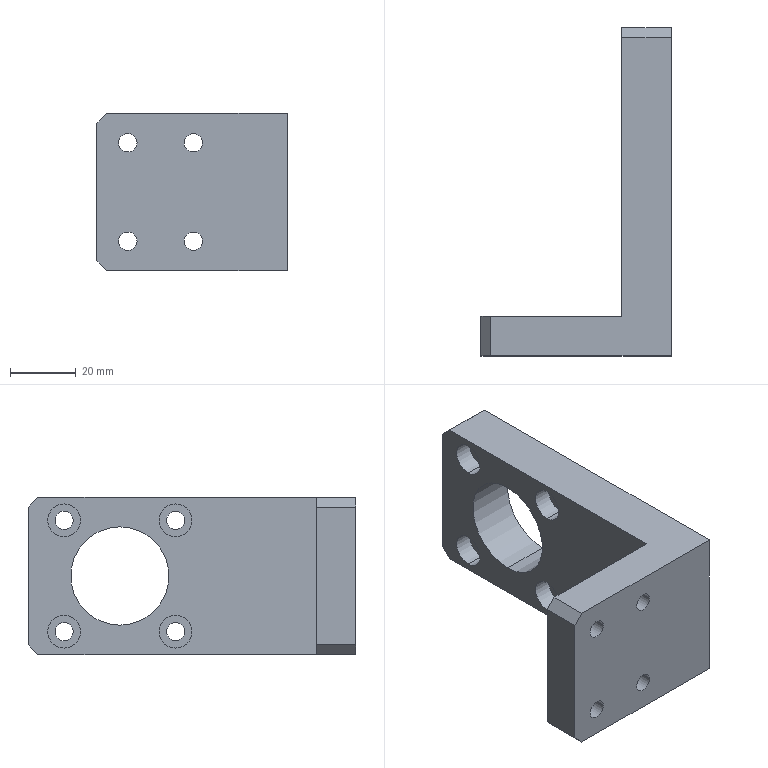Part | SolidWorks | features ICE 2, Chamfer 1, Extrusion 1, HoleWzd 1 | 1 solid | 42 faces | box 58 x 100 x 48 mm | volume 82065 mm3 | cylinder 26 | plane 16 | commonest cylinder face diameters 5.5 x8 5.6 x8 10 x8 30 x2
STEP:
#1=CARTESIAN_POINT('',(-20.01,-33.853,9.));
#2=VERTEX_POINT('',#1);
#3=CARTESIAN_POINT('',(-25.61,-33.853,9.));
#4=VERTEX_POINT('',#3);
#5=CARTESIAN_POINT('',(-22.81,-33.853,9.));
#6=DIRECTION('',(0.,1.,0.));
#7=DIRECTION('',(0.,0.,1.));
#8=AXIS2_PLACEMENT_3D('',#5,#6,#7);
#9=CIRCLE('',#8,2.8);
#10=EDGE_CURVE('',#2,#4,#9,.T.);
#11=ORIENTED_EDGE('',*,*,#10,.F.);
#12=CARTESIAN_POINT('',(-20.01,-21.853,9.));
#13=VERTEX_POINT('',#12);
#14=CARTESIAN_POINT('',(-20.01,-69.853,9.));
#15=DIRECTION('',(0.,1.,0.));
#16=VECTOR('',#15,1000.);
#17=LINE('',#14,#16);
#18=EDGE_CURVE('',#2,#13,#17,.T.);
#19=ORIENTED_EDGE('',*,*,#18,.T.);
#20=CARTESIAN_POINT('',(-25.61,-21.853,9.));
#21=VERTEX_POINT('',#20);
#22=CARTESIAN_POINT('',(-22.81,-21.853,9.));
#23=DIRECTION('',(0.,1.,0.));
#24=DIRECTION('',(-1.,0.,0.));
#25=AXIS2_PLACEMENT_3D('',#22,#23,#24);
#26=CIRCLE('',#25,2.8);
#27=EDGE_CURVE('',#13,#21,#26,.T.);
#28=ORIENTED_EDGE('',*,*,#27,.T.);
#29=CARTESIAN_POINT('',(-25.61,-69.853,9.));
#30=DIRECTION('',(0.,1.,0.));
#31=VECTOR('',#30,1000.);
#32=LINE('',#29,#31);
#33=EDGE_CURVE('',#4,#21,#32,.T.);
#34=ORIENTED_EDGE('',*,*,#33,.F.);
#35=EDGE_LOOP('',(#11,#19,#28,#34));
#36=FACE_OUTER_BOUND('',#35,.T.);
#37=CARTESIAN_POINT('',(-22.81,-69.853,9.));
#38=DIRECTION('',(0.,1.,0.));
#39=DIRECTION('',(-1.,0.,0.));
#40=AXIS2_PLACEMENT_3D('',#37,#38,#39);
#41=CYLINDRICAL_SURFACE('',#40,2.8);
#42=ADVANCED_FACE('',(#36),#41,.F.);
#43=CARTESIAN_POINT('',(-40.01,-33.853,39.));
#44=VERTEX_POINT('',#43);
#45=CARTESIAN_POINT('',(-45.61,-33.853,39.));
#46=VERTEX_POINT('',#45);
#47=CARTESIAN_POINT('',(-42.81,-33.853,39.));
#48=DIRECTION('',(0.,1.,0.));
#49=DIRECTION('',(0.,0.,1.));
#50=AXIS2_PLACEMENT_3D('',#47,#48,#49);
#51=CIRCLE('',#50,2.8);
#52=EDGE_CURVE('',#44,#46,#51,.T.);
#53=ORIENTED_EDGE('',*,*,#52,.F.);
#54=CARTESIAN_POINT('',(-40.01,-21.853,39.));
#55=VERTEX_POINT('',#54);
#56=CARTESIAN_POINT('',(-40.01,-69.853,39.));
#57=DIRECTION('',(0.,1.,0.));
#58=VECTOR('',#57,1000.);
#59=LINE('',#56,#58);
#60=EDGE_CURVE('',#44,#55,#59,.T.);
#61=ORIENTED_EDGE('',*,*,#60,.T.);
#62=CARTESIAN_POINT('',(-45.61,-21.853,39.));
#63=VERTEX_POINT('',#62);
#64=CARTESIAN_POINT('',(-42.81,-21.853,39.));
#65=DIRECTION('',(0.,1.,0.));
#66=DIRECTION('',(-1.,0.,0.));
#67=AXIS2_PLACEMENT_3D('',#64,#65,#66);
#68=CIRCLE('',#67,2.8);
#69=EDGE_CURVE('',#55,#63,#68,.T.);
#70=ORIENTED_EDGE('',*,*,#69,.T.);
#71=CARTESIAN_POINT('',(-45.61,-69.853,39.));
#72=DIRECTION('',(0.,1.,0.));
#73=VECTOR('',#72,1000.);
#74=LINE('',#71,#73);
#75=EDGE_CURVE('',#46,#63,#74,.T.);
#76=ORIENTED_EDGE('',*,*,#75,.F.);
#77=EDGE_LOOP('',(#53,#61,#70,#76));
#78=FACE_OUTER_BOUND('',#77,.T.);
#79=CARTESIAN_POINT('',(-42.81,-69.853,39.));
#80=DIRECTION('',(0.,1.,0.));
#81=DIRECTION('',(-1.,0.,0.));
#82=AXIS2_PLACEMENT_3D('',#79,#80,#81);
#83=CYLINDRICAL_SURFACE('',#82,2.8);
#84=ADVANCED_FACE('',(#78),#83,.F.);
#85=CARTESIAN_POINT('',(-20.01,-33.853,39.));
#86=VERTEX_POINT('',#85);
#87=CARTESIAN_POINT('',(-25.61,-33.853,39.));
#88=VERTEX_POINT('',#87);
#89=CARTESIAN_POINT('',(-22.81,-33.853,39.));
#90=DIRECTION('',(0.,1.,0.));
#91=DIRECTION('',(0.,0.,1.));
#92=AXIS2_PLACEMENT_3D('',#89,#90,#91);
#93=CIRCLE('',#92,2.8);
#94=EDGE_CURVE('',#86,#88,#93,.T.);
#95=ORIENTED_EDGE('',*,*,#94,.F.);
#96=CARTESIAN_POINT('',(-20.01,-21.853,39.));
#97=VERTEX_POINT('',#96);
#98=CARTESIAN_POINT('',(-20.01,-69.853,39.));
#99=DIRECTION('',(0.,1.,0.));
#100=VECTOR('',#99,1000.);
#101=LINE('',#98,#100);
#102=EDGE_CURVE('',#86,#97,#101,.T.);
#103=ORIENTED_EDGE('',*,*,#102,.T.);
#104=CARTESIAN_POINT('',(-25.61,-21.853,39.));
#105=VERTEX_POINT('',#104);
#106=CARTESIAN_POINT('',(-22.81,-21.853,39.));
#107=DIRECTION('',(0.,1.,0.));
#108=DIRECTION('',(-1.,0.,0.));
#109=AXIS2_PLACEMENT_3D('',#106,#107,#108);
#110=CIRCLE('',#109,2.8);
#111=EDGE_CURVE('',#97,#105,#110,.T.);
#112=ORIENTED_EDGE('',*,*,#111,.T.);
#113=CARTESIAN_POINT('',(-25.61,-69.853,39.));
#114=DIRECTION('',(0.,1.,0.));
#115=VECTOR('',#114,1000.);
#116=LINE('',#113,#115);
#117=EDGE_CURVE('',#88,#105,#116,.T.);
#118=ORIENTED_EDGE('',*,*,#117,.F.);
#119=EDGE_LOOP('',(#95,#103,#112,#118));
#120=FACE_OUTER_BOUND('',#119,.T.);
#121=CARTESIAN_POINT('',(-22.81,-69.853,39.));
#122=DIRECTION('',(0.,1.,0.));
#123=DIRECTION('',(-1.,0.,0.));
#124=AXIS2_PLACEMENT_3D('',#121,#122,#123);
#125=CYLINDRICAL_SURFACE('',#124,2.8);
#126=ADVANCED_FACE('',(#120),#125,.F.);
#127=CARTESIAN_POINT('',(-40.01,-33.853,9.));
#128=VERTEX_POINT('',#127);
#129=CARTESIAN_POINT('',(-45.61,-33.853,9.));
#130=VERTEX_POINT('',#129);
#131=CARTESIAN_POINT('',(-42.81,-33.853,9.));
#132=DIRECTION('',(0.,1.,0.));
#133=DIRECTION('',(0.,0.,1.));
#134=AXIS2_PLACEMENT_3D('',#131,#132,#133);
#135=CIRCLE('',#134,2.8);
#136=EDGE_CURVE('',#128,#130,#135,.T.);
#137=ORIENTED_EDGE('',*,*,#136,.F.);
#138=CARTESIAN_POINT('',(-40.01,-21.853,9.));
#139=VERTEX_POINT('',#138);
#140=CARTESIAN_POINT('',(-40.01,-69.853,9.));
#141=DIRECTION('',(0.,1.,0.));
#142=VECTOR('',#141,1000.);
#143=LINE('',#140,#142);
#144=EDGE_CURVE('',#128,#139,#143,.T.);
#145=ORIENTED_EDGE('',*,*,#144,.T.);
#146=CARTESIAN_POINT('',(-45.61,-21.853,9.));
#147=VERTEX_POINT('',#146);
#148=CARTESIAN_POINT('',(-42.81,-21.853,9.));
#149=DIRECTION('',(0.,1.,0.));
#150=DIRECTION('',(-1.,0.,0.));
#151=AXIS2_PLACEMENT_3D('',#148,#149,#150);
#152=CIRCLE('',#151,2.8);
#153=EDGE_CURVE('',#139,#147,#152,.T.);
#154=ORIENTED_EDGE('',*,*,#153,.T.);
#155=CARTESIAN_POINT('',(-45.61,-69.853,9.));
#156=DIRECTION('',(0.,1.,0.));
#157=VECTOR('',#156,1000.);
#158=LINE('',#155,#157);
#159=EDGE_CURVE('',#130,#147,#158,.T.);
#160=ORIENTED_EDGE('',*,*,#159,.F.);
#161=EDGE_LOOP('',(#137,#145,#154,#160));
#162=FACE_OUTER_BOUND('',#161,.T.);
#163=CARTESIAN_POINT('',(-42.81,-69.853,9.));
#164=DIRECTION('',(0.,1.,0.));
#165=DIRECTION('',(-1.,0.,0.));
#166=AXIS2_PLACEMENT_3D('',#163,#164,#165);
#167=CYLINDRICAL_SURFACE('',#166,2.8);
#168=ADVANCED_FACE('',(#162),#167,.F.);
#169=CARTESIAN_POINT('',(-3.547,55.147,2.));
#170=VERTEX_POINT('',#169);
#171=CARTESIAN_POINT('',(-3.547,55.147,12.));
#172=VERTEX_POINT('',#171);
#173=CARTESIAN_POINT('',(-3.547,55.147,7.));
#174=DIRECTION('',(-1.,0.,0.));
#175=DIRECTION('',(0.,0.,1.));
#176=AXIS2_PLACEMENT_3D('',#173,#174,#175);
#177=CIRCLE('',#176,5.);
#178=EDGE_CURVE('',#170,#172,#177,.T.);
#179=ORIENTED_EDGE('',*,*,#178,.F.);
#180=CARTESIAN_POINT('',(-9.247,55.147,2.));
#181=VERTEX_POINT('',#180);
#182=CARTESIAN_POINT('',(-9.247,55.147,2.));
#183=DIRECTION('',(-1.,0.,0.));
#184=VECTOR('',#183,1000.);
#185=LINE('',#182,#184);
#186=EDGE_CURVE('',#170,#181,#185,.T.);
#187=ORIENTED_EDGE('',*,*,#186,.T.);
#188=CARTESIAN_POINT('',(-9.247,55.147,12.));
#189=VERTEX_POINT('',#188);
#190=CARTESIAN_POINT('',(-9.247,55.147,7.));
#191=DIRECTION('',(-1.,0.,0.));
#192=DIRECTION('',(0.,0.,1.));
#193=AXIS2_PLACEMENT_3D('',#190,#191,#192);
#194=CIRCLE('',#193,5.);
#195=EDGE_CURVE('',#181,#189,#194,.T.);
#196=ORIENTED_EDGE('',*,*,#195,.T.);
#197=CARTESIAN_POINT('',(-9.247,55.147,12.));
#198=DIRECTION('',(-1.,0.,0.));
#199=VECTOR('',#198,1000.);
#200=LINE('',#197,#199);
#201=EDGE_CURVE('',#172,#189,#200,.T.);
#202=ORIENTED_EDGE('',*,*,#201,.F.);
#203=EDGE_LOOP('',(#179,#187,#196,#202));
#204=FACE_OUTER_BOUND('',#203,.T.);
#205=CARTESIAN_POINT('',(-9.247,55.147,7.));
#206=DIRECTION('',(-1.,0.,0.));
#207=DIRECTION('',(0.,0.,1.));
#208=AXIS2_PLACEMENT_3D('',#205,#206,#207);
#209=CYLINDRICAL_SURFACE('',#208,5.);
#210=ADVANCED_FACE('',(#204),#209,.F.);
#211=CARTESIAN_POINT('',(5.753,55.147,4.25));
#212=VERTEX_POINT('',#211);
#213=CARTESIAN_POINT('',(5.753,55.147,9.75));
#214=VERTEX_POINT('',#213);
#215=CARTESIAN_POINT('',(5.753,55.147,7.));
#216=DIRECTION('',(-1.,0.,0.));
#217=DIRECTION('',(0.,0.,1.));
#218=AXIS2_PLACEMENT_3D('',#215,#216,#217);
#219=CIRCLE('',#218,2.75);
#220=EDGE_CURVE('',#212,#214,#219,.T.);
#221=ORIENTED_EDGE('',*,*,#220,.F.);
#222=CARTESIAN_POINT('',(-3.547,55.147,4.25));
#223=VERTEX_POINT('',#222);
#224=CARTESIAN_POINT('',(-9.247,55.147,4.25));
#225=DIRECTION('',(-1.,0.,0.));
#226=VECTOR('',#225,1000.);
#227=LINE('',#224,#226);
#228=EDGE_CURVE('',#212,#223,#227,.T.);
#229=ORIENTED_EDGE('',*,*,#228,.T.);
#230=CARTESIAN_POINT('',(-3.547,55.147,9.75));
#231=VERTEX_POINT('',#230);
#232=CARTESIAN_POINT('',(-3.547,55.147,7.));
#233=DIRECTION('',(-1.,0.,0.));
#234=DIRECTION('',(0.,0.,1.));
#235=AXIS2_PLACEMENT_3D('',#232,#233,#234);
#236=CIRCLE('',#235,2.75);
#237=EDGE_CURVE('',#223,#231,#236,.T.);
#238=ORIENTED_EDGE('',*,*,#237,.T.);
#239=CARTESIAN_POINT('',(-9.247,55.147,9.75));
#240=DIRECTION('',(-1.,0.,0.));
#241=VECTOR('',#240,1000.);
#242=LINE('',#239,#241);
#243=EDGE_CURVE('',#214,#231,#242,.T.);
#244=ORIENTED_EDGE('',*,*,#243,.F.);
#245=EDGE_LOOP('',(#221,#229,#238,#244));
#246=FACE_OUTER_BOUND('',#245,.T.);
#247=CARTESIAN_POINT('',(-9.247,55.147,7.));
#248=DIRECTION('',(-1.,0.,0.));
#249=DIRECTION('',(0.,0.,1.));
#250=AXIS2_PLACEMENT_3D('',#247,#248,#249);
#251=CYLINDRICAL_SURFACE('',#250,2.75);
#252=ADVANCED_FACE('',(#246),#251,.F.);
#253=CARTESIAN_POINT('',(-3.547,55.147,36.));
#254=VERTEX_POINT('',#253);
#255=CARTESIAN_POINT('',(-3.547,55.147,46.));
#256=VERTEX_POINT('',#255);
#257=CARTESIAN_POINT('',(-3.547,55.147,41.));
#258=DIRECTION('',(-1.,0.,0.));
#259=DIRECTION('',(0.,0.,1.));
#260=AXIS2_PLACEMENT_3D('',#257,#258,#259);
#261=CIRCLE('',#260,5.);
#262=EDGE_CURVE('',#254,#256,#261,.T.);
#263=ORIENTED_EDGE('',*,*,#262,.F.);
#264=CARTESIAN_POINT('',(-9.247,55.147,36.));
#265=VERTEX_POINT('',#264);
#266=CARTESIAN_POINT('',(-9.247,55.147,36.));
#267=DIRECTION('',(-1.,0.,0.));
#268=VECTOR('',#267,1000.);
#269=LINE('',#266,#268);
#270=EDGE_CURVE('',#254,#265,#269,.T.);
#271=ORIENTED_EDGE('',*,*,#270,.T.);
#272=CARTESIAN_POINT('',(-9.247,55.147,46.));
#273=VERTEX_POINT('',#272);
#274=CARTESIAN_POINT('',(-9.247,55.147,41.));
#275=DIRECTION('',(-1.,0.,0.));
#276=DIRECTION('',(0.,0.,1.));
#277=AXIS2_PLACEMENT_3D('',#274,#275,#276);
#278=CIRCLE('',#277,5.);
#279=EDGE_CURVE('',#265,#273,#278,.T.);
#280=ORIENTED_EDGE('',*,*,#279,.T.);
#281=CARTESIAN_POINT('',(-9.247,55.147,46.));
#282=DIRECTION('',(-1.,0.,0.));
#283=VECTOR('',#282,1000.);
#284=LINE('',#281,#283);
#285=EDGE_CURVE('',#256,#273,#284,.T.);
#286=ORIENTED_EDGE('',*,*,#285,.F.);
#287=EDGE_LOOP('',(#263,#271,#280,#286));
#288=FACE_OUTER_BOUND('',#287,.T.);
#289=CARTESIAN_POINT('',(-9.247,55.147,41.));
#290=DIRECTION('',(-1.,0.,0.));
#291=DIRECTION('',(0.,0.,1.));
#292=AXIS2_PLACEMENT_3D('',#289,#290,#291);
#293=CYLINDRICAL_SURFACE('',#292,5.);
#294=ADVANCED_FACE('',(#288),#293,.F.);
#295=CARTESIAN_POINT('',(5.753,55.147,38.25));
#296=VERTEX_POINT('',#295);
#297=CARTESIAN_POINT('',(5.753,55.147,43.75));
#298=VERTEX_POINT('',#297);
#299=CARTESIAN_POINT('',(5.753,55.147,41.));
#300=DIRECTION('',(-1.,0.,0.));
#301=DIRECTION('',(0.,0.,1.));
#302=AXIS2_PLACEMENT_3D('',#299,#300,#301);
#303=CIRCLE('',#302,2.75);
#304=EDGE_CURVE('',#296,#298,#303,.T.);
#305=ORIENTED_EDGE('',*,*,#304,.F.);
#306=CARTESIAN_POINT('',(-3.547,55.147,38.25));
#307=VERTEX_POINT('',#306);
#308=CARTESIAN_POINT('',(-9.247,55.147,38.25));
#309=DIRECTION('',(-1.,0.,0.));
#310=VECTOR('',#309,1000.);
#311=LINE('',#308,#310);
#312=EDGE_CURVE('',#296,#307,#311,.T.);
#313=ORIENTED_EDGE('',*,*,#312,.T.);
#314=CARTESIAN_POINT('',(-3.547,55.147,43.75));
#315=VERTEX_POINT('',#314);
#316=CARTESIAN_POINT('',(-3.547,55.147,41.));
#317=DIRECTION('',(-1.,0.,0.));
#318=DIRECTION('',(0.,0.,1.));
#319=AXIS2_PLACEMENT_3D('',#316,#317,#318);
#320=CIRCLE('',#319,2.75);
#321=EDGE_CURVE('',#307,#315,#320,.T.);
#322=ORIENTED_EDGE('',*,*,#321,.T.);
#323=CARTESIAN_POINT('',(-9.247,55.147,43.75));
#324=DIRECTION('',(-1.,0.,0.));
#325=VECTOR('',#324,1000.);
#326=LINE('',#323,#325);
#327=EDGE_CURVE('',#298,#315,#326,.T.);
#328=ORIENTED_EDGE('',*,*,#327,.F.);
#329=EDGE_LOOP('',(#305,#313,#322,#328));
#330=FACE_OUTER_BOUND('',#329,.T.);
#331=CARTESIAN_POINT('',(-9.247,55.147,41.));
#332=DIRECTION('',(-1.,0.,0.));
#333=DIRECTION('',(0.,0.,1.));
#334=AXIS2_PLACEMENT_3D('',#331,#332,#333);
#335=CYLINDRICAL_SURFACE('',#334,2.75);
#336=ADVANCED_FACE('',(#330),#335,.F.);
#337=CARTESIAN_POINT('',(-3.547,21.147,36.));
#338=VERTEX_POINT('',#337);
#339=CARTESIAN_POINT('',(-3.547,21.147,46.));
#340=VERTEX_POINT('',#339);
#341=CARTESIAN_POINT('',(-3.547,21.147,41.));
#342=DIRECTION('',(-1.,0.,0.));
#343=DIRECTION('',(0.,0.,1.));
#344=AXIS2_PLACEMENT_3D('',#341,#342,#343);
#345=CIRCLE('',#344,5.);
#346=EDGE_CURVE('',#338,#340,#345,.T.);
#347=ORIENTED_EDGE('',*,*,#346,.F.);
#348=CARTESIAN_POINT('',(-9.247,21.147,36.));
#349=VERTEX_POINT('',#348);
#350=CARTESIAN_POINT('',(-9.247,21.147,36.));
#351=DIRECTION('',(-1.,0.,0.));
#352=VECTOR('',#351,1000.);
#353=LINE('',#350,#352);
#354=EDGE_CURVE('',#338,#349,#353,.T.);
#355=ORIENTED_EDGE('',*,*,#354,.T.);
#356=CARTESIAN_POINT('',(-9.247,21.147,46.));
#357=VERTEX_POINT('',#356);
#358=CARTESIAN_POINT('',(-9.247,21.147,41.));
#359=DIRECTION('',(-1.,0.,0.));
#360=DIRECTION('',(0.,0.,1.));
#361=AXIS2_PLACEMENT_3D('',#358,#359,#360);
#362=CIRCLE('',#361,5.);
#363=EDGE_CURVE('',#349,#357,#362,.T.);
#364=ORIENTED_EDGE('',*,*,#363,.T.);
#365=CARTESIAN_POINT('',(-9.247,21.147,46.));
#366=DIRECTION('',(-1.,0.,0.));
#367=VECTOR('',#366,1000.);
#368=LINE('',#365,#367);
#369=EDGE_CURVE('',#340,#357,#368,.T.);
#370=ORIENTED_EDGE('',*,*,#369,.F.);
#371=EDGE_LOOP('',(#347,#355,#364,#370));
#372=FACE_OUTER_BOUND('',#371,.T.);
#373=CARTESIAN_POINT('',(-9.247,21.147,41.));
#374=DIRECTION('',(-1.,0.,0.));
#375=DIRECTION('',(0.,0.,1.));
#376=AXIS2_PLACEMENT_3D('',#373,#374,#375);
#377=CYLINDRICAL_SURFACE('',#376,5.);
#378=ADVANCED_FACE('',(#372),#377,.F.);
#379=CARTESIAN_POINT('',(5.753,21.147,38.25));
#380=VERTEX_POINT('',#379);
#381=CARTESIAN_POINT('',(5.753,21.147,43.75));
#382=VERTEX_POINT('',#381);
#383=CARTESIAN_POINT('',(5.753,21.147,41.));
#384=DIRECTION('',(-1.,0.,0.));
#385=DIRECTION('',(0.,0.,1.));
#386=AXIS2_PLACEMENT_3D('',#383,#384,#385);
#387=CIRCLE('',#386,2.75);
#388=EDGE_CURVE('',#380,#382,#387,.T.);
#389=ORIENTED_EDGE('',*,*,#388,.F.);
#390=CARTESIAN_POINT('',(-3.547,21.147,38.25));
#391=VERTEX_POINT('',#390);
#392=CARTESIAN_POINT('',(-9.247,21.147,38.25));
#393=DIRECTION('',(-1.,0.,0.));
#394=VECTOR('',#393,1000.);
#395=LINE('',#392,#394);
#396=EDGE_CURVE('',#380,#391,#395,.T.);
#397=ORIENTED_EDGE('',*,*,#396,.T.);
#398=CARTESIAN_POINT('',(-3.547,21.147,43.75));
#399=VERTEX_POINT('',#398);
#400=CARTESIAN_POINT('',(-3.547,21.147,41.));
#401=DIRECTION('',(-1.,0.,0.));
#402=DIRECTION('',(0.,0.,1.));
#403=AXIS2_PLACEMENT_3D('',#400,#401,#402);
#404=CIRCLE('',#403,2.75);
#405=EDGE_CURVE('',#391,#399,#404,.T.);
#406=ORIENTED_EDGE('',*,*,#405,.T.);
#407=CARTESIAN_POINT('',(-9.247,21.147,43.75));
#408=DIRECTION('',(-1.,0.,0.));
#409=VECTOR('',#408,1000.);
#410=LINE('',#407,#409);
#411=EDGE_CURVE('',#382,#399,#410,.T.);
#412=ORIENTED_EDGE('',*,*,#411,.F.);
#413=EDGE_LOOP('',(#389,#397,#406,#412));
#414=FACE_OUTER_BOUND('',#413,.T.);
#415=CARTESIAN_POINT('',(-9.247,21.147,41.));
#416=DIRECTION('',(-1.,0.,0.));
#417=DIRECTION('',(0.,0.,1.));
#418=AXIS2_PLACEMENT_3D('',#415,#416,#417);
#419=CYLINDRICAL_SURFACE('',#418,2.75);
#420=ADVANCED_FACE('',(#414),#419,.F.);
#421=CARTESIAN_POINT('',(-3.547,21.147,2.));
#422=VERTEX_POINT('',#421);
#423=CARTESIAN_POINT('',(-3.547,21.147,12.));
#424=VERTEX_POINT('',#423);
#425=CARTESIAN_POINT('',(-3.547,21.147,7.));
#426=DIRECTION('',(-1.,0.,0.));
#427=DIRECTION('',(0.,0.,1.));
#428=AXIS2_PLACEMENT_3D('',#425,#426,#427);
#429=CIRCLE('',#428,5.);
#430=EDGE_CURVE('',#422,#424,#429,.T.);
#431=ORIENTED_EDGE('',*,*,#430,.F.);
#432=CARTESIAN_POINT('',(-9.247,21.147,2.));
#433=VERTEX_POINT('',#432);
#434=CARTESIAN_POINT('',(-9.247,21.147,2.));
#435=DIRECTION('',(-1.,0.,0.));
#436=VECTOR('',#435,1000.);
#437=LINE('',#434,#436);
#438=EDGE_CURVE('',#422,#433,#437,.T.);
#439=ORIENTED_EDGE('',*,*,#438,.T.);
#440=CARTESIAN_POINT('',(-9.247,21.147,12.));
#441=VERTEX_POINT('',#440);
#442=CARTESIAN_POINT('',(-9.247,21.147,7.));
#443=DIRECTION('',(-1.,0.,0.));
#444=DIRECTION('',(0.,0.,1.));
#445=AXIS2_PLACEMENT_3D('',#442,#443,#444);
#446=CIRCLE('',#445,5.);
#447=EDGE_CURVE('',#433,#441,#446,.T.);
#448=ORIENTED_EDGE('',*,*,#447,.T.);
#449=CARTESIAN_POINT('',(-9.247,21.147,12.));
#450=DIRECTION('',(-1.,0.,0.));
#451=VECTOR('',#450,1000.);
#452=LINE('',#449,#451);
#453=EDGE_CURVE('',#424,#441,#452,.T.);
#454=ORIENTED_EDGE('',*,*,#453,.F.);
#455=EDGE_LOOP('',(#431,#439,#448,#454));
#456=FACE_OUTER_BOUND('',#455,.T.);
#457=CARTESIAN_POINT('',(-9.247,21.147,7.));
#458=DIRECTION('',(-1.,0.,0.));
#459=DIRECTION('',(0.,0.,1.));
#460=AXIS2_PLACEMENT_3D('',#457,#458,#459);
#461=CYLINDRICAL_SURFACE('',#460,5.);
#462=ADVANCED_FACE('',(#456),#461,.F.);
#463=CARTESIAN_POINT('',(5.753,21.147,4.25));
#464=VERTEX_POINT('',#463);
#465=CARTESIAN_POINT('',(5.753,21.147,9.75));
#466=VERTEX_POINT('',#465);
#467=CARTESIAN_POINT('',(5.753,21.147,7.));
#468=DIRECTION('',(-1.,0.,0.));
#469=DIRECTION('',(0.,0.,1.));
#470=AXIS2_PLACEMENT_3D('',#467,#468,#469);
#471=CIRCLE('',#470,2.75);
#472=EDGE_CURVE('',#464,#466,#471,.T.);
#473=ORIENTED_EDGE('',*,*,#472,.F.);
#474=CARTESIAN_POINT('',(-3.547,21.147,4.25));
#475=VERTEX_POINT('',#474);
#476=CARTESIAN_POINT('',(-9.247,21.147,4.25));
#477=DIRECTION('',(-1.,0.,0.));
#478=VECTOR('',#477,1000.);
#479=LINE('',#476,#478);
#480=EDGE_CURVE('',#464,#475,#479,.T.);
#481=ORIENTED_EDGE('',*,*,#480,.T.);
#482=CARTESIAN_POINT('',(-3.547,21.147,9.75));
#483=VERTEX_POINT('',#482);
#484=CARTESIAN_POINT('',(-3.547,21.147,7.));
#485=DIRECTION('',(-1.,0.,0.));
#486=DIRECTION('',(0.,0.,1.));
#487=AXIS2_PLACEMENT_3D('',#484,#485,#486);
#488=CIRCLE('',#487,2.75);
#489=EDGE_CURVE('',#475,#483,#488,.T.);
#490=ORIENTED_EDGE('',*,*,#489,.T.);
#491=CARTESIAN_POINT('',(-9.247,21.147,9.75));
#492=DIRECTION('',(-1.,0.,0.));
#493=VECTOR('',#492,1000.);
#494=LINE('',#491,#493);
#495=EDGE_CURVE('',#466,#483,#494,.T.);
#496=ORIENTED_EDGE('',*,*,#495,.F.);
#497=EDGE_LOOP('',(#473,#481,#490,#496));
#498=FACE_OUTER_BOUND('',#497,.T.);
#499=CARTESIAN_POINT('',(-9.247,21.147,7.));
#500=DIRECTION('',(-1.,0.,0.));
#501=DIRECTION('',(0.,0.,1.));
#502=AXIS2_PLACEMENT_3D('',#499,#500,#501);
#503=CYLINDRICAL_SURFACE('',#502,2.75);
#504=ADVANCED_FACE('',(#498),#503,.F.);
#505=CARTESIAN_POINT('',(5.753,38.147,9.));
#506=VERTEX_POINT('',#505);
#507=CARTESIAN_POINT('',(5.753,38.147,39.));
#508=VERTEX_POINT('',#507);
#509=CARTESIAN_POINT('',(5.753,38.147,24.));
#510=DIRECTION('',(-1.,0.,0.));
#511=DIRECTION('',(0.,0.,1.));
#512=AXIS2_PLACEMENT_3D('',#509,#510,#511);
#513=CIRCLE('',#512,15.);
#514=EDGE_CURVE('',#506,#508,#513,.T.);
#515=ORIENTED_EDGE('',*,*,#514,.F.);
#516=CARTESIAN_POINT('',(-9.247,38.147,9.));
#517=VERTEX_POINT('',#516);
#518=CARTESIAN_POINT('',(5.753,38.147,9.));
#519=DIRECTION('',(-1.,0.,0.));
#520=VECTOR('',#519,1000.);
#521=LINE('',#518,#520);
#522=EDGE_CURVE('',#506,#517,#521,.T.);
#523=ORIENTED_EDGE('',*,*,#522,.T.);
#524=CARTESIAN_POINT('',(-9.247,38.147,39.));
#525=VERTEX_POINT('',#524);
#526=CARTESIAN_POINT('',(-9.247,38.147,24.));
#527=DIRECTION('',(-1.,0.,0.));
#528=DIRECTION('',(0.,0.,1.));
#529=AXIS2_PLACEMENT_3D('',#526,#527,#528);
#530=CIRCLE('',#529,15.);
#531=EDGE_CURVE('',#517,#525,#530,.T.);
#532=ORIENTED_EDGE('',*,*,#531,.T.);
#533=CARTESIAN_POINT('',(5.753,38.147,39.));
#534=DIRECTION('',(-1.,0.,0.));
#535=VECTOR('',#534,1000.);
#536=LINE('',#533,#535);
#537=EDGE_CURVE('',#508,#525,#536,.T.);
#538=ORIENTED_EDGE('',*,*,#537,.F.);
#539=EDGE_LOOP('',(#515,#523,#532,#538));
#540=FACE_OUTER_BOUND('',#539,.T.);
#541=CARTESIAN_POINT('',(5.753,38.147,24.));
#542=DIRECTION('',(-1.,0.,0.));
#543=DIRECTION('',(0.,0.,1.));
#544=AXIS2_PLACEMENT_3D('',#541,#542,#543);
#545=CYLINDRICAL_SURFACE('',#544,15.);
#546=ADVANCED_FACE('',(#540),#545,.F.);
#547=CARTESIAN_POINT('',(-9.247,66.147,45.));
#548=VERTEX_POINT('',#547);
#549=CARTESIAN_POINT('',(-9.247,66.147,3.));
#550=VERTEX_POINT('',#549);
#551=CARTESIAN_POINT('',(-9.247,66.147,48.));
#552=DIRECTION('',(0.,0.,-1.));
#553=VECTOR('',#552,1000.);
#554=LINE('',#551,#553);
#555=EDGE_CURVE('',#548,#550,#554,.T.);
#556=ORIENTED_EDGE('',*,*,#555,.F.);
#557=CARTESIAN_POINT('',(5.753,66.147,45.));
#558=VERTEX_POINT('',#557);
#559=CARTESIAN_POINT('',(5.753,66.147,45.));
#560=DIRECTION('',(1.,0.,0.));
#561=VECTOR('',#560,1000.);
#562=LINE('',#559,#561);
#563=EDGE_CURVE('',#548,#558,#562,.T.);
#564=ORIENTED_EDGE('',*,*,#563,.T.);
#565=CARTESIAN_POINT('',(5.753,66.147,3.));
#566=VERTEX_POINT('',#565);
#567=CARTESIAN_POINT('',(5.753,66.147,48.));
#568=DIRECTION('',(0.,0.,-1.));
#569=VECTOR('',#568,1000.);
#570=LINE('',#567,#569);
#571=EDGE_CURVE('',#558,#566,#570,.T.);
#572=ORIENTED_EDGE('',*,*,#571,.T.);
#573=CARTESIAN_POINT('',(5.753,66.147,3.));
#574=DIRECTION('',(-1.,0.,0.));
#575=VECTOR('',#574,1000.);
#576=LINE('',#573,#575);
#577=EDGE_CURVE('',#566,#550,#576,.T.);
#578=ORIENTED_EDGE('',*,*,#577,.T.);
#579=EDGE_LOOP('',(#556,#564,#572,#578));
#580=FACE_OUTER_BOUND('',#579,.T.);
#581=CARTESIAN_POINT('',(5.753,66.147,48.));
#582=DIRECTION('',(0.,-1.,0.));
#583=DIRECTION('',(0.,0.,-1.));
#584=AXIS2_PLACEMENT_3D('',#581,#582,#583);
#585=PLANE('',#584);
#586=ADVANCED_FACE('',(#580),#585,.F.);
#587=CARTESIAN_POINT('',(-9.247,55.147,7.));
#588=DIRECTION('',(-1.,0.,0.));
#589=DIRECTION('',(0.,0.,1.));
#590=AXIS2_PLACEMENT_3D('',#587,#588,#589);
#591=CIRCLE('',#590,5.);
#592=EDGE_CURVE('',#189,#181,#591,.T.);
#593=ORIENTED_EDGE('',*,*,#592,.F.);
#594=ORIENTED_EDGE('',*,*,#195,.F.);
#595=EDGE_LOOP('',(#593,#594));
#596=FACE_BOUND('',#595,.T.);
#597=CARTESIAN_POINT('',(-9.247,55.147,41.));
#598=DIRECTION('',(-1.,0.,0.));
#599=DIRECTION('',(0.,0.,1.));
#600=AXIS2_PLACEMENT_3D('',#597,#598,#599);
#601=CIRCLE('',#600,5.);
#602=EDGE_CURVE('',#273,#265,#601,.T.);
#603=ORIENTED_EDGE('',*,*,#602,.F.);
#604=ORIENTED_EDGE('',*,*,#279,.F.);
#605=EDGE_LOOP('',(#603,#604));
#606=FACE_BOUND('',#605,.T.);
#607=CARTESIAN_POINT('',(-9.247,21.147,41.));
#608=DIRECTION('',(-1.,0.,0.));
#609=DIRECTION('',(0.,0.,1.));
#610=AXIS2_PLACEMENT_3D('',#607,#608,#609);
#611=CIRCLE('',#610,5.);
#612=EDGE_CURVE('',#357,#349,#611,.T.);
#613=ORIENTED_EDGE('',*,*,#612,.F.);
#614=ORIENTED_EDGE('',*,*,#363,.F.);
#615=EDGE_LOOP('',(#613,#614));
#616=FACE_BOUND('',#615,.T.);
#617=CARTESIAN_POINT('',(-9.247,21.147,7.));
#618=DIRECTION('',(-1.,0.,0.));
#619=DIRECTION('',(0.,0.,1.));
#620=AXIS2_PLACEMENT_3D('',#617,#618,#619);
#621=CIRCLE('',#620,5.);
#622=EDGE_CURVE('',#441,#433,#621,.T.);
#623=ORIENTED_EDGE('',*,*,#622,.F.);
#624=ORIENTED_EDGE('',*,*,#447,.F.);
#625=EDGE_LOOP('',(#623,#624));
#626=FACE_BOUND('',#625,.T.);
#627=CARTESIAN_POINT('',(-9.247,38.147,24.));
#628=DIRECTION('',(-1.,0.,0.));
#629=DIRECTION('',(0.,0.,1.));
#630=AXIS2_PLACEMENT_3D('',#627,#628,#629);
#631=CIRCLE('',#630,15.);
#632=EDGE_CURVE('',#525,#517,#631,.T.);
#633=ORIENTED_EDGE('',*,*,#632,.F.);
#634=ORIENTED_EDGE('',*,*,#531,.F.);
#635=EDGE_LOOP('',(#633,#634));
#636=FACE_BOUND('',#635,.T.);
#637=CARTESIAN_POINT('',(-9.247,63.147,48.));
#638=VERTEX_POINT('',#637);
#639=CARTESIAN_POINT('',(-9.247,-21.853,48.));
#640=VERTEX_POINT('',#639);
#641=CARTESIAN_POINT('',(-9.247,66.147,48.));
#642=DIRECTION('',(0.,-1.,0.));
#643=VECTOR('',#642,1000.);
#644=LINE('',#641,#643);
#645=EDGE_CURVE('',#638,#640,#644,.T.);
#646=ORIENTED_EDGE('',*,*,#645,.F.);
#647=CARTESIAN_POINT('',(-9.247,63.147,48.));
#648=DIRECTION('',(0.,0.7071,-0.7071));
#649=VECTOR('',#648,1000.);
#650=LINE('',#647,#649);
#651=EDGE_CURVE('',#638,#548,#650,.T.);
#652=ORIENTED_EDGE('',*,*,#651,.T.);
#653=ORIENTED_EDGE('',*,*,#555,.T.);
#654=CARTESIAN_POINT('',(-9.247,63.147,0.));
#655=VERTEX_POINT('',#654);
#656=CARTESIAN_POINT('',(-9.247,66.147,3.));
#657=DIRECTION('',(0.,-0.7071,-0.7071));
#658=VECTOR('',#657,1000.);
#659=LINE('',#656,#658);
#660=EDGE_CURVE('',#550,#655,#659,.T.);
#661=ORIENTED_EDGE('',*,*,#660,.T.);
#662=CARTESIAN_POINT('',(-9.247,-21.853,0.));
#663=VERTEX_POINT('',#662);
#664=CARTESIAN_POINT('',(-9.247,66.147,0.));
#665=DIRECTION('',(0.,-1.,0.));
#666=VECTOR('',#665,1000.);
#667=LINE('',#664,#666);
#668=EDGE_CURVE('',#655,#663,#667,.T.);
#669=ORIENTED_EDGE('',*,*,#668,.T.);
#670=CARTESIAN_POINT('',(-9.247,-21.853,48.));
#671=DIRECTION('',(0.,0.,-1.));
#672=VECTOR('',#671,1000.);
#673=LINE('',#670,#672);
#674=EDGE_CURVE('',#640,#663,#673,.T.);
#675=ORIENTED_EDGE('',*,*,#674,.F.);
#676=EDGE_LOOP('',(#646,#652,#653,#661,#669,#675));
#677=FACE_OUTER_BOUND('',#676,.T.);
#678=CARTESIAN_POINT('',(-9.247,66.147,48.));
#679=DIRECTION('',(1.,0.,0.));
#680=DIRECTION('',(0.,0.,-1.));
#681=AXIS2_PLACEMENT_3D('',#678,#679,#680);
#682=PLANE('',#681);
#683=ADVANCED_FACE('',(#596,#606,#616,#626,#636,#677),#682,.F.);
#684=CARTESIAN_POINT('',(-22.81,-21.853,9.));
#685=DIRECTION('',(0.,1.,0.));
#686=DIRECTION('',(-1.,0.,0.));
#687=AXIS2_PLACEMENT_3D('',#684,#685,#686);
#688=CIRCLE('',#687,2.8);
#689=EDGE_CURVE('',#21,#13,#688,.T.);
#690=ORIENTED_EDGE('',*,*,#689,.F.);
#691=ORIENTED_EDGE('',*,*,#27,.F.);
#692=EDGE_LOOP('',(#690,#691));
#693=FACE_BOUND('',#692,.T.);
#694=CARTESIAN_POINT('',(-42.81,-21.853,39.));
#695=DIRECTION('',(0.,1.,0.));
#696=DIRECTION('',(-1.,0.,0.));
#697=AXIS2_PLACEMENT_3D('',#694,#695,#696);
#698=CIRCLE('',#697,2.8);
#699=EDGE_CURVE('',#63,#55,#698,.T.);
#700=ORIENTED_EDGE('',*,*,#699,.F.);
#701=ORIENTED_EDGE('',*,*,#69,.F.);
#702=EDGE_LOOP('',(#700,#701));
#703=FACE_BOUND('',#702,.T.);
#704=CARTESIAN_POINT('',(-22.81,-21.853,39.));
#705=DIRECTION('',(0.,1.,0.));
#706=DIRECTION('',(-1.,0.,0.));
#707=AXIS2_PLACEMENT_3D('',#704,#705,#706);
#708=CIRCLE('',#707,2.8);
#709=EDGE_CURVE('',#105,#97,#708,.T.);
#710=ORIENTED_EDGE('',*,*,#709,.F.);
#711=ORIENTED_EDGE('',*,*,#111,.F.);
#712=EDGE_LOOP('',(#710,#711));
#713=FACE_BOUND('',#712,.T.);
#714=CARTESIAN_POINT('',(-42.81,-21.853,9.));
#715=DIRECTION('',(0.,1.,0.));
#716=DIRECTION('',(-1.,0.,0.));
#717=AXIS2_PLACEMENT_3D('',#714,#715,#716);
#718=CIRCLE('',#717,2.8);
#719=EDGE_CURVE('',#147,#139,#718,.T.);
#720=ORIENTED_EDGE('',*,*,#719,.F.);
#721=ORIENTED_EDGE('',*,*,#153,.F.);
#722=EDGE_LOOP('',(#720,#721));
#723=FACE_BOUND('',#722,.T.);
#724=CARTESIAN_POINT('',(-52.247,-21.853,45.));
#725=VERTEX_POINT('',#724);
#726=CARTESIAN_POINT('',(-52.247,-21.853,3.));
#727=VERTEX_POINT('',#726);
#728=CARTESIAN_POINT('',(-52.247,-21.853,48.));
#729=DIRECTION('',(0.,0.,-1.));
#730=VECTOR('',#729,1000.);
#731=LINE('',#728,#730);
#732=EDGE_CURVE('',#725,#727,#731,.T.);
#733=ORIENTED_EDGE('',*,*,#732,.F.);
#734=CARTESIAN_POINT('',(-49.247,-21.853,48.));
#735=VERTEX_POINT('',#734);
#736=CARTESIAN_POINT('',(-49.247,-21.853,48.));
#737=DIRECTION('',(0.7071,0.,0.7071));
#738=VECTOR('',#737,1000.);
#739=LINE('',#736,#738);
#740=EDGE_CURVE('',#725,#735,#739,.T.);
#741=ORIENTED_EDGE('',*,*,#740,.T.);
#742=CARTESIAN_POINT('',(-9.247,-21.853,48.));
#743=DIRECTION('',(-1.,0.,0.));
#744=VECTOR('',#743,1000.);
#745=LINE('',#742,#744);
#746=EDGE_CURVE('',#640,#735,#745,.T.);
#747=ORIENTED_EDGE('',*,*,#746,.F.);
#748=ORIENTED_EDGE('',*,*,#674,.T.);
#749=CARTESIAN_POINT('',(-49.247,-21.853,0.));
#750=VERTEX_POINT('',#749);
#751=CARTESIAN_POINT('',(-9.247,-21.853,0.));
#752=DIRECTION('',(-1.,0.,0.));
#753=VECTOR('',#752,1000.);
#754=LINE('',#751,#753);
#755=EDGE_CURVE('',#663,#750,#754,.T.);
#756=ORIENTED_EDGE('',*,*,#755,.T.);
#757=CARTESIAN_POINT('',(-52.247,-21.853,3.));
#758=DIRECTION('',(-0.7071,0.,0.7071));
#759=VECTOR('',#758,1000.);
#760=LINE('',#757,#759);
#761=EDGE_CURVE('',#750,#727,#760,.T.);
#762=ORIENTED_EDGE('',*,*,#761,.T.);
#763=EDGE_LOOP('',(#733,#741,#747,#748,#756,#762));
#764=FACE_OUTER_BOUND('',#763,.T.);
#765=CARTESIAN_POINT('',(-9.247,-21.853,48.));
#766=DIRECTION('',(0.,-1.,0.));
#767=DIRECTION('',(1.,0.,0.));
#768=AXIS2_PLACEMENT_3D('',#765,#766,#767);
#769=PLANE('',#768);
#770=ADVANCED_FACE('',(#693,#703,#713,#723,#764),#769,.F.);
#771=CARTESIAN_POINT('',(-52.247,-33.853,45.));
#772=VERTEX_POINT('',#771);
#773=CARTESIAN_POINT('',(-52.247,-33.853,3.));
#774=VERTEX_POINT('',#773);
#775=CARTESIAN_POINT('',(-52.247,-33.853,48.));
#776=DIRECTION('',(0.,0.,-1.));
#777=VECTOR('',#776,1000.);
#778=LINE('',#775,#777);
#779=EDGE_CURVE('',#772,#774,#778,.T.);
#780=ORIENTED_EDGE('',*,*,#779,.F.);
#781=CARTESIAN_POINT('',(-52.247,-21.853,45.));
#782=DIRECTION('',(0.,1.,0.));
#783=VECTOR('',#782,1000.);
#784=LINE('',#781,#783);
#785=EDGE_CURVE('',#772,#725,#784,.T.);
#786=ORIENTED_EDGE('',*,*,#785,.T.);
#787=ORIENTED_EDGE('',*,*,#732,.T.);
#788=CARTESIAN_POINT('',(-52.247,-21.853,3.));
#789=DIRECTION('',(0.,-1.,0.));
#790=VECTOR('',#789,1000.);
#791=LINE('',#788,#790);
#792=EDGE_CURVE('',#727,#774,#791,.T.);
#793=ORIENTED_EDGE('',*,*,#792,.T.);
#794=EDGE_LOOP('',(#780,#786,#787,#793));
#795=FACE_OUTER_BOUND('',#794,.T.);
#796=CARTESIAN_POINT('',(-52.247,-21.853,48.));
#797=DIRECTION('',(1.,0.,0.));
#798=DIRECTION('',(0.,0.,-1.));
#799=AXIS2_PLACEMENT_3D('',#796,#797,#798);
#800=PLANE('',#799);
#801=ADVANCED_FACE('',(#795),#800,.F.);
#802=CARTESIAN_POINT('',(-22.81,-33.853,9.));
#803=DIRECTION('',(0.,1.,0.));
#804=DIRECTION('',(0.,0.,1.));
#805=AXIS2_PLACEMENT_3D('',#802,#803,#804);
#806=CIRCLE('',#805,2.8);
#807=EDGE_CURVE('',#4,#2,#806,.T.);
#808=ORIENTED_EDGE('',*,*,#807,.T.);
#809=ORIENTED_EDGE('',*,*,#10,.T.);
#810=EDGE_LOOP('',(#808,#809));
#811=FACE_BOUND('',#810,.T.);
#812=CARTESIAN_POINT('',(-42.81,-33.853,39.));
#813=DIRECTION('',(0.,1.,0.));
#814=DIRECTION('',(0.,0.,1.));
#815=AXIS2_PLACEMENT_3D('',#812,#813,#814);
#816=CIRCLE('',#815,2.8);
#817=EDGE_CURVE('',#46,#44,#816,.T.);
#818=ORIENTED_EDGE('',*,*,#817,.T.);
#819=ORIENTED_EDGE('',*,*,#52,.T.);
#820=EDGE_LOOP('',(#818,#819));
#821=FACE_BOUND('',#820,.T.);
#822=CARTESIAN_POINT('',(-22.81,-33.853,39.));
#823=DIRECTION('',(0.,1.,0.));
#824=DIRECTION('',(0.,0.,1.));
#825=AXIS2_PLACEMENT_3D('',#822,#823,#824);
#826=CIRCLE('',#825,2.8);
#827=EDGE_CURVE('',#88,#86,#826,.T.);
#828=ORIENTED_EDGE('',*,*,#827,.T.);
#829=ORIENTED_EDGE('',*,*,#94,.T.);
#830=EDGE_LOOP('',(#828,#829));
#831=FACE_BOUND('',#830,.T.);
#832=CARTESIAN_POINT('',(-42.81,-33.853,9.));
#833=DIRECTION('',(0.,1.,0.));
#834=DIRECTION('',(0.,0.,1.));
#835=AXIS2_PLACEMENT_3D('',#832,#833,#834);
#836=CIRCLE('',#835,2.8);
#837=EDGE_CURVE('',#130,#128,#836,.T.);
#838=ORIENTED_EDGE('',*,*,#837,.T.);
#839=ORIENTED_EDGE('',*,*,#136,.T.);
#840=EDGE_LOOP('',(#838,#839));
#841=FACE_BOUND('',#840,.T.);
#842=CARTESIAN_POINT('',(-49.247,-33.853,48.));
#843=VERTEX_POINT('',#842);
#844=CARTESIAN_POINT('',(5.753,-33.853,48.));
#845=VERTEX_POINT('',#844);
#846=CARTESIAN_POINT('',(-52.247,-33.853,48.));
#847=DIRECTION('',(1.,0.,0.));
#848=VECTOR('',#847,1000.);
#849=LINE('',#846,#848);
#850=EDGE_CURVE('',#843,#845,#849,.T.);
#851=ORIENTED_EDGE('',*,*,#850,.F.);
#852=CARTESIAN_POINT('',(-49.247,-33.853,48.));
#853=DIRECTION('',(-0.7071,0.,-0.7071));
#854=VECTOR('',#853,1000.);
#855=LINE('',#852,#854);
#856=EDGE_CURVE('',#843,#772,#855,.T.);
#857=ORIENTED_EDGE('',*,*,#856,.T.);
#858=ORIENTED_EDGE('',*,*,#779,.T.);
#859=CARTESIAN_POINT('',(-49.247,-33.853,0.));
#860=VERTEX_POINT('',#859);
#861=CARTESIAN_POINT('',(-52.247,-33.853,3.));
#862=DIRECTION('',(0.7071,0.,-0.7071));
#863=VECTOR('',#862,1000.);
#864=LINE('',#861,#863);
#865=EDGE_CURVE('',#774,#860,#864,.T.);
#866=ORIENTED_EDGE('',*,*,#865,.T.);
#867=CARTESIAN_POINT('',(5.753,-33.853,0.));
#868=VERTEX_POINT('',#867);
#869=CARTESIAN_POINT('',(-52.247,-33.853,0.));
#870=DIRECTION('',(1.,0.,0.));
#871=VECTOR('',#870,1000.);
#872=LINE('',#869,#871);
#873=EDGE_CURVE('',#860,#868,#872,.T.);
#874=ORIENTED_EDGE('',*,*,#873,.T.);
#875=CARTESIAN_POINT('',(5.753,-33.853,48.));
#876=DIRECTION('',(0.,0.,-1.));
#877=VECTOR('',#876,1000.);
#878=LINE('',#875,#877);
#879=EDGE_CURVE('',#845,#868,#878,.T.);
#880=ORIENTED_EDGE('',*,*,#879,.F.);
#881=EDGE_LOOP('',(#851,#857,#858,#866,#874,#880));
#882=FACE_OUTER_BOUND('',#881,.T.);
#883=CARTESIAN_POINT('',(-52.247,-33.853,48.));
#884=DIRECTION('',(0.,1.,0.));
#885=DIRECTION('',(0.,0.,1.));
#886=AXIS2_PLACEMENT_3D('',#883,#884,#885);
#887=PLANE('',#886);
#888=ADVANCED_FACE('',(#811,#821,#831,#841,#882),#887,.F.);
#889=CARTESIAN_POINT('',(5.753,55.147,7.));
#890=DIRECTION('',(-1.,0.,0.));
#891=DIRECTION('',(0.,0.,1.));
#892=AXIS2_PLACEMENT_3D('',#889,#890,#891);
#893=CIRCLE('',#892,2.75);
#894=EDGE_CURVE('',#214,#212,#893,.T.);
#895=ORIENTED_EDGE('',*,*,#894,.T.);
#896=ORIENTED_EDGE('',*,*,#220,.T.);
#897=EDGE_LOOP('',(#895,#896));
#898=FACE_BOUND('',#897,.T.);
#899=CARTESIAN_POINT('',(5.753,55.147,41.));
#900=DIRECTION('',(-1.,0.,0.));
#901=DIRECTION('',(0.,0.,1.));
#902=AXIS2_PLACEMENT_3D('',#899,#900,#901);
#903=CIRCLE('',#902,2.75);
#904=EDGE_CURVE('',#298,#296,#903,.T.);
#905=ORIENTED_EDGE('',*,*,#904,.T.);
#906=ORIENTED_EDGE('',*,*,#304,.T.);
#907=EDGE_LOOP('',(#905,#906));
#908=FACE_BOUND('',#907,.T.);
#909=CARTESIAN_POINT('',(5.753,21.147,41.));
#910=DIRECTION('',(-1.,0.,0.));
#911=DIRECTION('',(0.,0.,1.));
#912=AXIS2_PLACEMENT_3D('',#909,#910,#911);
#913=CIRCLE('',#912,2.75);
#914=EDGE_CURVE('',#382,#380,#913,.T.);
#915=ORIENTED_EDGE('',*,*,#914,.T.);
#916=ORIENTED_EDGE('',*,*,#388,.T.);
#917=EDGE_LOOP('',(#915,#916));
#918=FACE_BOUND('',#917,.T.);
#919=CARTESIAN_POINT('',(5.753,21.147,7.));
#920=DIRECTION('',(-1.,0.,0.));
#921=DIRECTION('',(0.,0.,1.));
#922=AXIS2_PLACEMENT_3D('',#919,#920,#921);
#923=CIRCLE('',#922,2.75);
#924=EDGE_CURVE('',#466,#464,#923,.T.);
#925=ORIENTED_EDGE('',*,*,#924,.T.);
#926=ORIENTED_EDGE('',*,*,#472,.T.);
#927=EDGE_LOOP('',(#925,#926));
#928=FACE_BOUND('',#927,.T.);
#929=CARTESIAN_POINT('',(5.753,38.147,24.));
#930=DIRECTION('',(-1.,0.,0.));
#931=DIRECTION('',(0.,0.,1.));
#932=AXIS2_PLACEMENT_3D('',#929,#930,#931);
#933=CIRCLE('',#932,15.);
#934=EDGE_CURVE('',#508,#506,#933,.T.);
#935=ORIENTED_EDGE('',*,*,#934,.T.);
#936=ORIENTED_EDGE('',*,*,#514,.T.);
#937=EDGE_LOOP('',(#935,#936));
#938=FACE_BOUND('',#937,.T.);
#939=ORIENTED_EDGE('',*,*,#571,.F.);
#940=CARTESIAN_POINT('',(5.753,63.147,48.));
#941=VERTEX_POINT('',#940);
#942=CARTESIAN_POINT('',(5.753,63.147,48.));
#943=DIRECTION('',(0.,-0.7071,0.7071));
#944=VECTOR('',#943,1000.);
#945=LINE('',#942,#944);
#946=EDGE_CURVE('',#558,#941,#945,.T.);
#947=ORIENTED_EDGE('',*,*,#946,.T.);
#948=CARTESIAN_POINT('',(5.753,-33.853,48.));
#949=DIRECTION('',(0.,1.,0.));
#950=VECTOR('',#949,1000.);
#951=LINE('',#948,#950);
#952=EDGE_CURVE('',#845,#941,#951,.T.);
#953=ORIENTED_EDGE('',*,*,#952,.F.);
#954=ORIENTED_EDGE('',*,*,#879,.T.);
#955=CARTESIAN_POINT('',(5.753,63.147,0.));
#956=VERTEX_POINT('',#955);
#957=CARTESIAN_POINT('',(5.753,-33.853,0.));
#958=DIRECTION('',(0.,1.,0.));
#959=VECTOR('',#958,1000.);
#960=LINE('',#957,#959);
#961=EDGE_CURVE('',#868,#956,#960,.T.);
#962=ORIENTED_EDGE('',*,*,#961,.T.);
#963=CARTESIAN_POINT('',(5.753,66.147,3.));
#964=DIRECTION('',(0.,0.7071,0.7071));
#965=VECTOR('',#964,1000.);
#966=LINE('',#963,#965);
#967=EDGE_CURVE('',#956,#566,#966,.T.);
#968=ORIENTED_EDGE('',*,*,#967,.T.);
#969=EDGE_LOOP('',(#939,#947,#953,#954,#962,#968));
#970=FACE_OUTER_BOUND('',#969,.T.);
#971=CARTESIAN_POINT('',(5.753,-33.853,48.));
#972=DIRECTION('',(-1.,0.,0.));
#973=DIRECTION('',(0.,-1.,0.));
#974=AXIS2_PLACEMENT_3D('',#971,#972,#973);
#975=PLANE('',#974);
#976=ADVANCED_FACE('',(#898,#908,#918,#928,#938,#970),#975,.F.);
#977=ORIENTED_EDGE('',*,*,#746,.T.);
#978=CARTESIAN_POINT('',(-49.247,-33.853,48.));
#979=DIRECTION('',(0.,-1.,0.));
#980=VECTOR('',#979,1000.);
#981=LINE('',#978,#980);
#982=EDGE_CURVE('',#735,#843,#981,.T.);
#983=ORIENTED_EDGE('',*,*,#982,.T.);
#984=ORIENTED_EDGE('',*,*,#850,.T.);
#985=ORIENTED_EDGE('',*,*,#952,.T.);
#986=CARTESIAN_POINT('',(-9.247,63.147,48.));
#987=DIRECTION('',(-1.,0.,0.));
#988=VECTOR('',#987,1000.);
#989=LINE('',#986,#988);
#990=EDGE_CURVE('',#941,#638,#989,.T.);
#991=ORIENTED_EDGE('',*,*,#990,.T.);
#992=ORIENTED_EDGE('',*,*,#645,.T.);
#993=EDGE_LOOP('',(#977,#983,#984,#985,#991,#992));
#994=FACE_OUTER_BOUND('',#993,.T.);
#995=CARTESIAN_POINT('',(0.,0.,48.));
#996=DIRECTION('',(0.,0.,1.));
#997=DIRECTION('',(1.,0.,0.));
#998=AXIS2_PLACEMENT_3D('',#995,#996,#997);
#999=PLANE('',#998);
#1000=ADVANCED_FACE('',(#994),#999,.T.);
#1001=ORIENTED_EDGE('',*,*,#873,.F.);
#1002=CARTESIAN_POINT('',(-49.247,0.,0.));
#1003=DIRECTION('',(0.,1.,0.));
#1004=VECTOR('',#1003,1000.);
#1005=LINE('',#1002,#1004);
#1006=EDGE_CURVE('',#860,#750,#1005,.T.);
#1007=ORIENTED_EDGE('',*,*,#1006,.T.);
#1008=ORIENTED_EDGE('',*,*,#755,.F.);
#1009=ORIENTED_EDGE('',*,*,#668,.F.);
#1010=CARTESIAN_POINT('',(0.,63.147,0.));
#1011=DIRECTION('',(1.,0.,0.));
#1012=VECTOR('',#1011,1000.);
#1013=LINE('',#1010,#1012);
#1014=EDGE_CURVE('',#655,#956,#1013,.T.);
#1015=ORIENTED_EDGE('',*,*,#1014,.T.);
#1016=ORIENTED_EDGE('',*,*,#961,.F.);
#1017=EDGE_LOOP('',(#1001,#1007,#1008,#1009,#1015,#1016));
#1018=FACE_OUTER_BOUND('',#1017,.T.);
#1019=CARTESIAN_POINT('',(0.,0.,0.));
#1020=DIRECTION('',(0.,0.,1.));
#1021=DIRECTION('',(1.,0.,0.));
#1022=AXIS2_PLACEMENT_3D('',#1019,#1020,#1021);
#1023=PLANE('',#1022);
#1024=ADVANCED_FACE('',(#1018),#1023,.F.);
#1025=ORIENTED_EDGE('',*,*,#522,.F.);
#1026=ORIENTED_EDGE('',*,*,#934,.F.);
#1027=ORIENTED_EDGE('',*,*,#537,.T.);
#1028=ORIENTED_EDGE('',*,*,#632,.T.);
#1029=EDGE_LOOP('',(#1025,#1026,#1027,#1028));
#1030=FACE_OUTER_BOUND('',#1029,.T.);
#1031=CARTESIAN_POINT('',(5.753,38.147,24.));
#1032=DIRECTION('',(-1.,0.,0.));
#1033=DIRECTION('',(0.,0.,1.));
#1034=AXIS2_PLACEMENT_3D('',#1031,#1032,#1033);
#1035=CYLINDRICAL_SURFACE('',#1034,15.);
#1036=ADVANCED_FACE('',(#1030),#1035,.F.);
#1037=ORIENTED_EDGE('',*,*,#480,.F.);
#1038=ORIENTED_EDGE('',*,*,#924,.F.);
#1039=ORIENTED_EDGE('',*,*,#495,.T.);
#1040=CARTESIAN_POINT('',(-3.547,21.147,7.));
#1041=DIRECTION('',(-1.,0.,0.));
#1042=DIRECTION('',(0.,0.,1.));
#1043=AXIS2_PLACEMENT_3D('',#1040,#1041,#1042);
#1044=CIRCLE('',#1043,2.75);
#1045=EDGE_CURVE('',#483,#475,#1044,.T.);
#1046=ORIENTED_EDGE('',*,*,#1045,.T.);
#1047=EDGE_LOOP('',(#1037,#1038,#1039,#1046));
#1048=FACE_OUTER_BOUND('',#1047,.T.);
#1049=CARTESIAN_POINT('',(-9.247,21.147,7.));
#1050=DIRECTION('',(-1.,0.,0.));
#1051=DIRECTION('',(0.,0.,1.));
#1052=AXIS2_PLACEMENT_3D('',#1049,#1050,#1051);
#1053=CYLINDRICAL_SURFACE('',#1052,2.75);
#1054=ADVANCED_FACE('',(#1048),#1053,.F.);
#1055=ORIENTED_EDGE('',*,*,#1045,.F.);
#1056=ORIENTED_EDGE('',*,*,#489,.F.);
#1057=EDGE_LOOP('',(#1055,#1056));
#1058=FACE_BOUND('',#1057,.T.);
#1059=CARTESIAN_POINT('',(-3.547,21.147,7.));
#1060=DIRECTION('',(-1.,0.,0.));
#1061=DIRECTION('',(0.,0.,1.));
#1062=AXIS2_PLACEMENT_3D('',#1059,#1060,#1061);
#1063=CIRCLE('',#1062,5.);
#1064=EDGE_CURVE('',#424,#422,#1063,.T.);
#1065=ORIENTED_EDGE('',*,*,#1064,.T.);
#1066=ORIENTED_EDGE('',*,*,#430,.T.);
#1067=EDGE_LOOP('',(#1065,#1066));
#1068=FACE_OUTER_BOUND('',#1067,.T.);
#1069=CARTESIAN_POINT('',(-3.547,23.897,7.));
#1070=DIRECTION('',(1.,0.,0.));
#1071=DIRECTION('',(0.,0.,-1.));
#1072=AXIS2_PLACEMENT_3D('',#1069,#1070,#1071);
#1073=PLANE('',#1072);
#1074=ADVANCED_FACE('',(#1058,#1068),#1073,.F.);
#1075=ORIENTED_EDGE('',*,*,#438,.F.);
#1076=ORIENTED_EDGE('',*,*,#1064,.F.);
#1077=ORIENTED_EDGE('',*,*,#453,.T.);
#1078=ORIENTED_EDGE('',*,*,#622,.T.);
#1079=EDGE_LOOP('',(#1075,#1076,#1077,#1078));
#1080=FACE_OUTER_BOUND('',#1079,.T.);
#1081=CARTESIAN_POINT('',(-9.247,21.147,7.));
#1082=DIRECTION('',(-1.,0.,0.));
#1083=DIRECTION('',(0.,0.,1.));
#1084=AXIS2_PLACEMENT_3D('',#1081,#1082,#1083);
#1085=CYLINDRICAL_SURFACE('',#1084,5.);
#1086=ADVANCED_FACE('',(#1080),#1085,.F.);
#1087=ORIENTED_EDGE('',*,*,#396,.F.);
#1088=ORIENTED_EDGE('',*,*,#914,.F.);
#1089=ORIENTED_EDGE('',*,*,#411,.T.);
#1090=CARTESIAN_POINT('',(-3.547,21.147,41.));
#1091=DIRECTION('',(-1.,0.,0.));
#1092=DIRECTION('',(0.,0.,1.));
#1093=AXIS2_PLACEMENT_3D('',#1090,#1091,#1092);
#1094=CIRCLE('',#1093,2.75);
#1095=EDGE_CURVE('',#399,#391,#1094,.T.);
#1096=ORIENTED_EDGE('',*,*,#1095,.T.);
#1097=EDGE_LOOP('',(#1087,#1088,#1089,#1096));
#1098=FACE_OUTER_BOUND('',#1097,.T.);
#1099=CARTESIAN_POINT('',(-9.247,21.147,41.));
#1100=DIRECTION('',(-1.,0.,0.));
#1101=DIRECTION('',(0.,0.,1.));
#1102=AXIS2_PLACEMENT_3D('',#1099,#1100,#1101);
#1103=CYLINDRICAL_SURFACE('',#1102,2.75);
#1104=ADVANCED_FACE('',(#1098),#1103,.F.);
#1105=ORIENTED_EDGE('',*,*,#1095,.F.);
#1106=ORIENTED_EDGE('',*,*,#405,.F.);
#1107=EDGE_LOOP('',(#1105,#1106));
#1108=FACE_BOUND('',#1107,.T.);
#1109=CARTESIAN_POINT('',(-3.547,21.147,41.));
#1110=DIRECTION('',(-1.,0.,0.));
#1111=DIRECTION('',(0.,0.,1.));
#1112=AXIS2_PLACEMENT_3D('',#1109,#1110,#1111);
#1113=CIRCLE('',#1112,5.);
#1114=EDGE_CURVE('',#340,#338,#1113,.T.);
#1115=ORIENTED_EDGE('',*,*,#1114,.T.);
#1116=ORIENTED_EDGE('',*,*,#346,.T.);
#1117=EDGE_LOOP('',(#1115,#1116));
#1118=FACE_OUTER_BOUND('',#1117,.T.);
#1119=CARTESIAN_POINT('',(-3.547,23.897,41.));
#1120=DIRECTION('',(1.,0.,0.));
#1121=DIRECTION('',(0.,0.,-1.));
#1122=AXIS2_PLACEMENT_3D('',#1119,#1120,#1121);
#1123=PLANE('',#1122);
#1124=ADVANCED_FACE('',(#1108,#1118),#1123,.F.);
#1125=ORIENTED_EDGE('',*,*,#354,.F.);
#1126=ORIENTED_EDGE('',*,*,#1114,.F.);
#1127=ORIENTED_EDGE('',*,*,#369,.T.);
#1128=ORIENTED_EDGE('',*,*,#612,.T.);
#1129=EDGE_LOOP('',(#1125,#1126,#1127,#1128));
#1130=FACE_OUTER_BOUND('',#1129,.T.);
#1131=CARTESIAN_POINT('',(-9.247,21.147,41.));
#1132=DIRECTION('',(-1.,0.,0.));
#1133=DIRECTION('',(0.,0.,1.));
#1134=AXIS2_PLACEMENT_3D('',#1131,#1132,#1133);
#1135=CYLINDRICAL_SURFACE('',#1134,5.);
#1136=ADVANCED_FACE('',(#1130),#1135,.F.);
#1137=ORIENTED_EDGE('',*,*,#312,.F.);
#1138=ORIENTED_EDGE('',*,*,#904,.F.);
#1139=ORIENTED_EDGE('',*,*,#327,.T.);
#1140=CARTESIAN_POINT('',(-3.547,55.147,41.));
#1141=DIRECTION('',(-1.,0.,0.));
#1142=DIRECTION('',(0.,0.,1.));
#1143=AXIS2_PLACEMENT_3D('',#1140,#1141,#1142);
#1144=CIRCLE('',#1143,2.75);
#1145=EDGE_CURVE('',#315,#307,#1144,.T.);
#1146=ORIENTED_EDGE('',*,*,#1145,.T.);
#1147=EDGE_LOOP('',(#1137,#1138,#1139,#1146));
#1148=FACE_OUTER_BOUND('',#1147,.T.);
#1149=CARTESIAN_POINT('',(-9.247,55.147,41.));
#1150=DIRECTION('',(-1.,0.,0.));
#1151=DIRECTION('',(0.,0.,1.));
#1152=AXIS2_PLACEMENT_3D('',#1149,#1150,#1151);
#1153=CYLINDRICAL_SURFACE('',#1152,2.75);
#1154=ADVANCED_FACE('',(#1148),#1153,.F.);
#1155=ORIENTED_EDGE('',*,*,#1145,.F.);
#1156=ORIENTED_EDGE('',*,*,#321,.F.);
#1157=EDGE_LOOP('',(#1155,#1156));
#1158=FACE_BOUND('',#1157,.T.);
#1159=CARTESIAN_POINT('',(-3.547,55.147,41.));
#1160=DIRECTION('',(-1.,0.,0.));
#1161=DIRECTION('',(0.,0.,1.));
#1162=AXIS2_PLACEMENT_3D('',#1159,#1160,#1161);
#1163=CIRCLE('',#1162,5.);
#1164=EDGE_CURVE('',#256,#254,#1163,.T.);
#1165=ORIENTED_EDGE('',*,*,#1164,.T.);
#1166=ORIENTED_EDGE('',*,*,#262,.T.);
#1167=EDGE_LOOP('',(#1165,#1166));
#1168=FACE_OUTER_BOUND('',#1167,.T.);
#1169=CARTESIAN_POINT('',(-3.547,57.897,41.));
#1170=DIRECTION('',(1.,0.,0.));
#1171=DIRECTION('',(0.,0.,-1.));
#1172=AXIS2_PLACEMENT_3D('',#1169,#1170,#1171);
#1173=PLANE('',#1172);
#1174=ADVANCED_FACE('',(#1158,#1168),#1173,.F.);
#1175=ORIENTED_EDGE('',*,*,#270,.F.);
#1176=ORIENTED_EDGE('',*,*,#1164,.F.);
#1177=ORIENTED_EDGE('',*,*,#285,.T.);
#1178=ORIENTED_EDGE('',*,*,#602,.T.);
#1179=EDGE_LOOP('',(#1175,#1176,#1177,#1178));
#1180=FACE_OUTER_BOUND('',#1179,.T.);
#1181=CARTESIAN_POINT('',(-9.247,55.147,41.));
#1182=DIRECTION('',(-1.,0.,0.));
#1183=DIRECTION('',(0.,0.,1.));
#1184=AXIS2_PLACEMENT_3D('',#1181,#1182,#1183);
#1185=CYLINDRICAL_SURFACE('',#1184,5.);
#1186=ADVANCED_FACE('',(#1180),#1185,.F.);
#1187=ORIENTED_EDGE('',*,*,#228,.F.);
#1188=ORIENTED_EDGE('',*,*,#894,.F.);
#1189=ORIENTED_EDGE('',*,*,#243,.T.);
#1190=CARTESIAN_POINT('',(-3.547,55.147,7.));
#1191=DIRECTION('',(-1.,0.,0.));
#1192=DIRECTION('',(0.,0.,1.));
#1193=AXIS2_PLACEMENT_3D('',#1190,#1191,#1192);
#1194=CIRCLE('',#1193,2.75);
#1195=EDGE_CURVE('',#231,#223,#1194,.T.);
#1196=ORIENTED_EDGE('',*,*,#1195,.T.);
#1197=EDGE_LOOP('',(#1187,#1188,#1189,#1196));
#1198=FACE_OUTER_BOUND('',#1197,.T.);
#1199=CARTESIAN_POINT('',(-9.247,55.147,7.));
#1200=DIRECTION('',(-1.,0.,0.));
#1201=DIRECTION('',(0.,0.,1.));
#1202=AXIS2_PLACEMENT_3D('',#1199,#1200,#1201);
#1203=CYLINDRICAL_SURFACE('',#1202,2.75);
#1204=ADVANCED_FACE('',(#1198),#1203,.F.);
#1205=ORIENTED_EDGE('',*,*,#1195,.F.);
#1206=ORIENTED_EDGE('',*,*,#237,.F.);
#1207=EDGE_LOOP('',(#1205,#1206));
#1208=FACE_BOUND('',#1207,.T.);
#1209=CARTESIAN_POINT('',(-3.547,55.147,7.));
#1210=DIRECTION('',(-1.,0.,0.));
#1211=DIRECTION('',(0.,0.,1.));
#1212=AXIS2_PLACEMENT_3D('',#1209,#1210,#1211);
#1213=CIRCLE('',#1212,5.);
#1214=EDGE_CURVE('',#172,#170,#1213,.T.);
#1215=ORIENTED_EDGE('',*,*,#1214,.T.);
#1216=ORIENTED_EDGE('',*,*,#178,.T.);
#1217=EDGE_LOOP('',(#1215,#1216));
#1218=FACE_OUTER_BOUND('',#1217,.T.);
#1219=CARTESIAN_POINT('',(-3.547,57.897,7.));
#1220=DIRECTION('',(1.,0.,0.));
#1221=DIRECTION('',(0.,0.,-1.));
#1222=AXIS2_PLACEMENT_3D('',#1219,#1220,#1221);
#1223=PLANE('',#1222);
#1224=ADVANCED_FACE('',(#1208,#1218),#1223,.F.);
#1225=ORIENTED_EDGE('',*,*,#186,.F.);
#1226=ORIENTED_EDGE('',*,*,#1214,.F.);
#1227=ORIENTED_EDGE('',*,*,#201,.T.);
#1228=ORIENTED_EDGE('',*,*,#592,.T.);
#1229=EDGE_LOOP('',(#1225,#1226,#1227,#1228));
#1230=FACE_OUTER_BOUND('',#1229,.T.);
#1231=CARTESIAN_POINT('',(-9.247,55.147,7.));
#1232=DIRECTION('',(-1.,0.,0.));
#1233=DIRECTION('',(0.,0.,1.));
#1234=AXIS2_PLACEMENT_3D('',#1231,#1232,#1233);
#1235=CYLINDRICAL_SURFACE('',#1234,5.);
#1236=ADVANCED_FACE('',(#1230),#1235,.F.);
#1237=ORIENTED_EDGE('',*,*,#740,.F.);
#1238=ORIENTED_EDGE('',*,*,#785,.F.);
#1239=ORIENTED_EDGE('',*,*,#856,.F.);
#1240=ORIENTED_EDGE('',*,*,#982,.F.);
#1241=EDGE_LOOP('',(#1237,#1238,#1239,#1240));
#1242=FACE_OUTER_BOUND('',#1241,.T.);
#1243=CARTESIAN_POINT('',(-49.247,0.,48.));
#1244=DIRECTION('',(-0.7071,0.,0.7071));
#1245=DIRECTION('',(0.,1.,0.));
#1246=AXIS2_PLACEMENT_3D('',#1243,#1244,#1245);
#1247=PLANE('',#1246);
#1248=ADVANCED_FACE('',(#1242),#1247,.T.);
#1249=ORIENTED_EDGE('',*,*,#761,.F.);
#1250=ORIENTED_EDGE('',*,*,#1006,.F.);
#1251=ORIENTED_EDGE('',*,*,#865,.F.);
#1252=ORIENTED_EDGE('',*,*,#792,.F.);
#1253=EDGE_LOOP('',(#1249,#1250,#1251,#1252));
#1254=FACE_OUTER_BOUND('',#1253,.T.);
#1255=CARTESIAN_POINT('',(-52.247,-21.853,3.));
#1256=DIRECTION('',(0.7071,0.,0.7071));
#1257=DIRECTION('',(0.,-1.,0.));
#1258=AXIS2_PLACEMENT_3D('',#1255,#1256,#1257);
#1259=PLANE('',#1258);
#1260=ADVANCED_FACE('',(#1254),#1259,.F.);
#1261=ORIENTED_EDGE('',*,*,#946,.F.);
#1262=ORIENTED_EDGE('',*,*,#563,.F.);
#1263=ORIENTED_EDGE('',*,*,#651,.F.);
#1264=ORIENTED_EDGE('',*,*,#990,.F.);
#1265=EDGE_LOOP('',(#1261,#1262,#1263,#1264));
#1266=FACE_OUTER_BOUND('',#1265,.T.);
#1267=CARTESIAN_POINT('',(0.,63.147,48.));
#1268=DIRECTION('',(0.,0.7071,0.7071));
#1269=DIRECTION('',(1.,0.,0.));
#1270=AXIS2_PLACEMENT_3D('',#1267,#1268,#1269);
#1271=PLANE('',#1270);
#1272=ADVANCED_FACE('',(#1266),#1271,.T.);
#1273=ORIENTED_EDGE('',*,*,#967,.F.);
#1274=ORIENTED_EDGE('',*,*,#1014,.F.);
#1275=ORIENTED_EDGE('',*,*,#660,.F.);
#1276=ORIENTED_EDGE('',*,*,#577,.F.);
#1277=EDGE_LOOP('',(#1273,#1274,#1275,#1276));
#1278=FACE_OUTER_BOUND('',#1277,.T.);
#1279=CARTESIAN_POINT('',(5.753,66.147,3.));
#1280=DIRECTION('',(0.,-0.7071,0.7071));
#1281=DIRECTION('',(-1.,0.,0.));
#1282=AXIS2_PLACEMENT_3D('',#1279,#1280,#1281);
#1283=PLANE('',#1282);
#1284=ADVANCED_FACE('',(#1278),#1283,.F.);
#1285=ORIENTED_EDGE('',*,*,#144,.F.);
#1286=ORIENTED_EDGE('',*,*,#837,.F.);
#1287=ORIENTED_EDGE('',*,*,#159,.T.);
#1288=ORIENTED_EDGE('',*,*,#719,.T.);
#1289=EDGE_LOOP('',(#1285,#1286,#1287,#1288));
#1290=FACE_OUTER_BOUND('',#1289,.T.);
#1291=CARTESIAN_POINT('',(-42.81,-69.853,9.));
#1292=DIRECTION('',(0.,1.,0.));
#1293=DIRECTION('',(-1.,0.,0.));
#1294=AXIS2_PLACEMENT_3D('',#1291,#1292,#1293);
#1295=CYLINDRICAL_SURFACE('',#1294,2.8);
#1296=ADVANCED_FACE('',(#1290),#1295,.F.);
#1297=ORIENTED_EDGE('',*,*,#102,.F.);
#1298=ORIENTED_EDGE('',*,*,#827,.F.);
#1299=ORIENTED_EDGE('',*,*,#117,.T.);
#1300=ORIENTED_EDGE('',*,*,#709,.T.);
#1301=EDGE_LOOP('',(#1297,#1298,#1299,#1300));
#1302=FACE_OUTER_BOUND('',#1301,.T.);
#1303=CARTESIAN_POINT('',(-22.81,-69.853,39.));
#1304=DIRECTION('',(0.,1.,0.));
#1305=DIRECTION('',(-1.,0.,0.));
#1306=AXIS2_PLACEMENT_3D('',#1303,#1304,#1305);
#1307=CYLINDRICAL_SURFACE('',#1306,2.8);
#1308=ADVANCED_FACE('',(#1302),#1307,.F.);
#1309=ORIENTED_EDGE('',*,*,#60,.F.);
#1310=ORIENTED_EDGE('',*,*,#817,.F.);
#1311=ORIENTED_EDGE('',*,*,#75,.T.);
#1312=ORIENTED_EDGE('',*,*,#699,.T.);
#1313=EDGE_LOOP('',(#1309,#1310,#1311,#1312));
#1314=FACE_OUTER_BOUND('',#1313,.T.);
#1315=CARTESIAN_POINT('',(-42.81,-69.853,39.));
#1316=DIRECTION('',(0.,1.,0.));
#1317=DIRECTION('',(-1.,0.,0.));
#1318=AXIS2_PLACEMENT_3D('',#1315,#1316,#1317);
#1319=CYLINDRICAL_SURFACE('',#1318,2.8);
#1320=ADVANCED_FACE('',(#1314),#1319,.F.);
#1321=ORIENTED_EDGE('',*,*,#18,.F.);
#1322=ORIENTED_EDGE('',*,*,#807,.F.);
#1323=ORIENTED_EDGE('',*,*,#33,.T.);
#1324=ORIENTED_EDGE('',*,*,#689,.T.);
#1325=EDGE_LOOP('',(#1321,#1322,#1323,#1324));
#1326=FACE_OUTER_BOUND('',#1325,.T.);
#1327=CARTESIAN_POINT('',(-22.81,-69.853,9.));
#1328=DIRECTION('',(0.,1.,0.));
#1329=DIRECTION('',(-1.,0.,0.));
#1330=AXIS2_PLACEMENT_3D('',#1327,#1328,#1329);
#1331=CYLINDRICAL_SURFACE('',#1330,2.8);
#1332=ADVANCED_FACE('',(#1326),#1331,.F.);
#1333=CLOSED_SHELL('',(#42,#84,#126,#168,#210,#252,#294,#336,#378,#420,#462,#504,#546,#586,#683,#770,#801,#888,#976,#1000,#1024,#1036,#1054,#1074,#1086,#1104,#1124,#1136,#1154,#1174,#1186,#1204,#1224,#1236,#1248,#1260,#1272,#1284,#1296,#1308,#1320,#1332));
#1334=MANIFOLD_SOLID_BREP('',#1333);
#1335=CARTESIAN_POINT('',(0.,0.,0.));
#1336=DIRECTION('',(0.,0.,1.));
#1337=DIRECTION('',(1.,0.,0.));
#1338=AXIS2_PLACEMENT_3D('',#1335,#1336,#1337);
#1339=(LENGTH_UNIT()NAMED_UNIT(*)SI_UNIT(.MILLI.,.METRE.));
#1340=UNCERTAINTY_MEASURE_WITH_UNIT(LENGTH_MEASURE(0.00001),#1339,'','');
#1341=(NAMED_UNIT(*)PLANE_ANGLE_UNIT()SI_UNIT($,.RADIAN.));
#1342=(NAMED_UNIT(*)SI_UNIT($,.STERADIAN.)SOLID_ANGLE_UNIT());
#1343=(GEOMETRIC_REPRESENTATION_CONTEXT(3)GLOBAL_UNCERTAINTY_ASSIGNED_CONTEXT((#1340))GLOBAL_UNIT_ASSIGNED_CONTEXT((#1339,#1341,#1342))REPRESENTATION_CONTEXT('',''));
#1344=ADVANCED_BREP_SHAPE_REPRESENTATION('',(#1334,#1338),#1343);